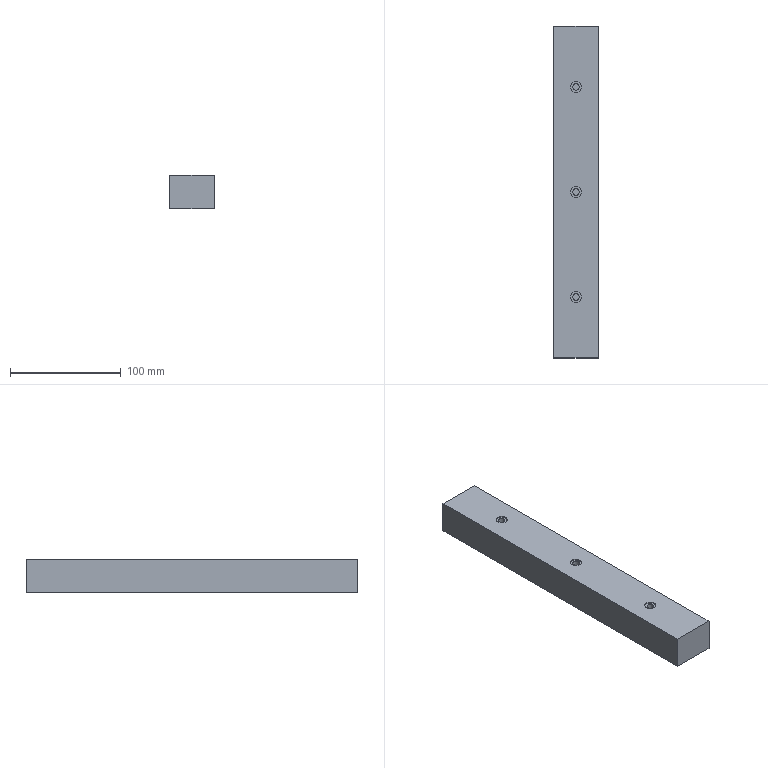Part | STEP file | lizhu | 1 solid | 18 faces | box 40 x 300 x 30 mm | volume 358407 mm3 | plane 12 | cylinder 6 | commonest cylinder face diameters 6 x3 10 x3
STEP:
#1=CARTESIAN_POINT('',(0.,0.,0.));
#2=DIRECTION('',(0.,0.,1.));
#3=DIRECTION('',(1.,0.,0.));
#4=AXIS2_PLACEMENT_3D('',#1,#2,#3);
#5=CARTESIAN_POINT('',(20.,-150.,0.));
#6=VERTEX_POINT('',#5);
#7=CARTESIAN_POINT('',(20.,150.,0.));
#8=VERTEX_POINT('',#7);
#9=CARTESIAN_POINT('',(20.,150.,0.));
#10=DIRECTION('',(0.,1.,0.));
#11=VECTOR('',#10,1.);
#12=LINE('',#9,#11);
#13=CARTESIAN_POINT('',(20.,150.,30.));
#14=DIRECTION('',(-1.,0.,0.));
#15=DIRECTION('',(0.,-1.,0.));
#16=AXIS2_PLACEMENT_3D('',#13,#14,#15);
#17=PLANE('',#16);
#18=CARTESIAN_POINT('',(0.,-30.));
#19=DIRECTION('',(-1.,0.));
#20=VECTOR('',#19,1.);
#21=LINE('',#18,#20);
#22=(GEOMETRIC_REPRESENTATION_CONTEXT(2)PARAMETRIC_REPRESENTATION_CONTEXT()REPRESENTATION_CONTEXT('',''));
#23=DEFINITIONAL_REPRESENTATION('',(#21),#22);
#24=PCURVE('',#17,#23);
#25=CARTESIAN_POINT('',(0.,0.,0.));
#26=DIRECTION('',(0.,0.,1.));
#27=DIRECTION('',(1.,0.,0.));
#28=AXIS2_PLACEMENT_3D('',#25,#26,#27);
#29=PLANE('',#28);
#30=CARTESIAN_POINT('',(20.,150.));
#31=DIRECTION('',(0.,1.));
#32=VECTOR('',#31,1.);
#33=LINE('',#30,#32);
#34=(GEOMETRIC_REPRESENTATION_CONTEXT(2)PARAMETRIC_REPRESENTATION_CONTEXT()REPRESENTATION_CONTEXT('',''));
#35=DEFINITIONAL_REPRESENTATION('',(#33),#34);
#36=PCURVE('',#29,#35);
#37=SURFACE_CURVE('',#12,(#24,#36),.PCURVE_S1.);
#38=EDGE_CURVE('',#6,#8,#37,.T.);
#39=ORIENTED_EDGE('',*,*,#38,.T.);
#40=CARTESIAN_POINT('',(20.,150.,30.));
#41=VERTEX_POINT('',#40);
#42=CARTESIAN_POINT('',(20.,150.,30.));
#43=DIRECTION('',(0.,0.,-1.));
#44=VECTOR('',#43,1.);
#45=LINE('',#42,#44);
#46=CARTESIAN_POINT('',(0.,0.));
#47=DIRECTION('',(0.,-1.));
#48=VECTOR('',#47,1.);
#49=LINE('',#46,#48);
#50=(GEOMETRIC_REPRESENTATION_CONTEXT(2)PARAMETRIC_REPRESENTATION_CONTEXT()REPRESENTATION_CONTEXT('',''));
#51=DEFINITIONAL_REPRESENTATION('',(#49),#50);
#52=PCURVE('',#17,#51);
#53=CARTESIAN_POINT('',(-20.,150.,30.));
#54=DIRECTION('',(0.,-1.,0.));
#55=DIRECTION('',(0.,0.,-1.));
#56=AXIS2_PLACEMENT_3D('',#53,#54,#55);
#57=PLANE('',#56);
#58=CARTESIAN_POINT('',(0.,40.));
#59=DIRECTION('',(1.,0.));
#60=VECTOR('',#59,1.);
#61=LINE('',#58,#60);
#62=(GEOMETRIC_REPRESENTATION_CONTEXT(2)PARAMETRIC_REPRESENTATION_CONTEXT()REPRESENTATION_CONTEXT('',''));
#63=DEFINITIONAL_REPRESENTATION('',(#61),#62);
#64=PCURVE('',#57,#63);
#65=SURFACE_CURVE('',#45,(#52,#64),.PCURVE_S1.);
#66=EDGE_CURVE('',#41,#8,#65,.T.);
#67=ORIENTED_EDGE('',*,*,#66,.F.);
#68=CARTESIAN_POINT('',(20.,-150.,30.));
#69=VERTEX_POINT('',#68);
#70=CARTESIAN_POINT('',(20.,150.,30.));
#71=DIRECTION('',(0.,1.,0.));
#72=VECTOR('',#71,1.);
#73=LINE('',#70,#72);
#74=CARTESIAN_POINT('',(0.,0.));
#75=DIRECTION('',(-1.,0.));
#76=VECTOR('',#75,1.);
#77=LINE('',#74,#76);
#78=(GEOMETRIC_REPRESENTATION_CONTEXT(2)PARAMETRIC_REPRESENTATION_CONTEXT()REPRESENTATION_CONTEXT('',''));
#79=DEFINITIONAL_REPRESENTATION('',(#77),#78);
#80=PCURVE('',#17,#79);
#81=CARTESIAN_POINT('',(0.,0.,30.));
#82=DIRECTION('',(0.,0.,1.));
#83=DIRECTION('',(1.,0.,0.));
#84=AXIS2_PLACEMENT_3D('',#81,#82,#83);
#85=PLANE('',#84);
#86=CARTESIAN_POINT('',(20.,150.));
#87=DIRECTION('',(0.,1.));
#88=VECTOR('',#87,1.);
#89=LINE('',#86,#88);
#90=(GEOMETRIC_REPRESENTATION_CONTEXT(2)PARAMETRIC_REPRESENTATION_CONTEXT()REPRESENTATION_CONTEXT('',''));
#91=DEFINITIONAL_REPRESENTATION('',(#89),#90);
#92=PCURVE('',#85,#91);
#93=SURFACE_CURVE('',#73,(#80,#92),.PCURVE_S1.);
#94=EDGE_CURVE('',#69,#41,#93,.T.);
#95=ORIENTED_EDGE('',*,*,#94,.F.);
#96=CARTESIAN_POINT('',(20.,-150.,30.));
#97=DIRECTION('',(0.,0.,-1.));
#98=VECTOR('',#97,1.);
#99=LINE('',#96,#98);
#100=CARTESIAN_POINT('',(300.,0.));
#101=DIRECTION('',(0.,-1.));
#102=VECTOR('',#101,1.);
#103=LINE('',#100,#102);
#104=(GEOMETRIC_REPRESENTATION_CONTEXT(2)PARAMETRIC_REPRESENTATION_CONTEXT()REPRESENTATION_CONTEXT('',''));
#105=DEFINITIONAL_REPRESENTATION('',(#103),#104);
#106=PCURVE('',#17,#105);
#107=CARTESIAN_POINT('',(-20.,-150.,30.));
#108=DIRECTION('',(0.,1.,0.));
#109=DIRECTION('',(0.,0.,1.));
#110=AXIS2_PLACEMENT_3D('',#107,#108,#109);
#111=PLANE('',#110);
#112=CARTESIAN_POINT('',(0.,40.));
#113=DIRECTION('',(-1.,0.));
#114=VECTOR('',#113,1.);
#115=LINE('',#112,#114);
#116=(GEOMETRIC_REPRESENTATION_CONTEXT(2)PARAMETRIC_REPRESENTATION_CONTEXT()REPRESENTATION_CONTEXT('',''));
#117=DEFINITIONAL_REPRESENTATION('',(#115),#116);
#118=PCURVE('',#111,#117);
#119=SURFACE_CURVE('',#99,(#106,#118),.PCURVE_S1.);
#120=EDGE_CURVE('',#69,#6,#119,.T.);
#121=ORIENTED_EDGE('',*,*,#120,.T.);
#122=EDGE_LOOP('',(#39,#67,#95,#121));
#123=FACE_BOUND('',#122,.T.);
#124=ADVANCED_FACE('',(#123),#17,.F.);
#125=CARTESIAN_POINT('',(-20.,150.,0.));
#126=VERTEX_POINT('',#125);
#127=CARTESIAN_POINT('',(-20.,150.,0.));
#128=DIRECTION('',(-1.,0.,0.));
#129=VECTOR('',#128,1.);
#130=LINE('',#127,#129);
#131=CARTESIAN_POINT('',(30.,0.));
#132=DIRECTION('',(0.,-1.));
#133=VECTOR('',#132,1.);
#134=LINE('',#131,#133);
#135=(GEOMETRIC_REPRESENTATION_CONTEXT(2)PARAMETRIC_REPRESENTATION_CONTEXT()REPRESENTATION_CONTEXT('',''));
#136=DEFINITIONAL_REPRESENTATION('',(#134),#135);
#137=PCURVE('',#57,#136);
#138=CARTESIAN_POINT('',(-20.,150.));
#139=DIRECTION('',(-1.,0.));
#140=VECTOR('',#139,1.);
#141=LINE('',#138,#140);
#142=(GEOMETRIC_REPRESENTATION_CONTEXT(2)PARAMETRIC_REPRESENTATION_CONTEXT()REPRESENTATION_CONTEXT('',''));
#143=DEFINITIONAL_REPRESENTATION('',(#141),#142);
#144=PCURVE('',#29,#143);
#145=SURFACE_CURVE('',#130,(#137,#144),.PCURVE_S1.);
#146=EDGE_CURVE('',#8,#126,#145,.T.);
#147=ORIENTED_EDGE('',*,*,#146,.T.);
#148=CARTESIAN_POINT('',(-20.,150.,30.));
#149=VERTEX_POINT('',#148);
#150=CARTESIAN_POINT('',(-20.,150.,30.));
#151=DIRECTION('',(0.,0.,-1.));
#152=VECTOR('',#151,1.);
#153=LINE('',#150,#152);
#154=CARTESIAN_POINT('',(0.,0.));
#155=DIRECTION('',(1.,0.));
#156=VECTOR('',#155,1.);
#157=LINE('',#154,#156);
#158=(GEOMETRIC_REPRESENTATION_CONTEXT(2)PARAMETRIC_REPRESENTATION_CONTEXT()REPRESENTATION_CONTEXT('',''));
#159=DEFINITIONAL_REPRESENTATION('',(#157),#158);
#160=PCURVE('',#57,#159);
#161=CARTESIAN_POINT('',(-20.,150.,30.));
#162=DIRECTION('',(1.,0.,0.));
#163=DIRECTION('',(0.,1.,0.));
#164=AXIS2_PLACEMENT_3D('',#161,#162,#163);
#165=PLANE('',#164);
#166=CARTESIAN_POINT('',(0.,0.));
#167=DIRECTION('',(0.,-1.));
#168=VECTOR('',#167,1.);
#169=LINE('',#166,#168);
#170=(GEOMETRIC_REPRESENTATION_CONTEXT(2)PARAMETRIC_REPRESENTATION_CONTEXT()REPRESENTATION_CONTEXT('',''));
#171=DEFINITIONAL_REPRESENTATION('',(#169),#170);
#172=PCURVE('',#165,#171);
#173=SURFACE_CURVE('',#153,(#160,#172),.PCURVE_S1.);
#174=EDGE_CURVE('',#149,#126,#173,.T.);
#175=ORIENTED_EDGE('',*,*,#174,.F.);
#176=CARTESIAN_POINT('',(-20.,150.,30.));
#177=DIRECTION('',(-1.,0.,0.));
#178=VECTOR('',#177,1.);
#179=LINE('',#176,#178);
#180=CARTESIAN_POINT('',(0.,0.));
#181=DIRECTION('',(0.,-1.));
#182=VECTOR('',#181,1.);
#183=LINE('',#180,#182);
#184=(GEOMETRIC_REPRESENTATION_CONTEXT(2)PARAMETRIC_REPRESENTATION_CONTEXT()REPRESENTATION_CONTEXT('',''));
#185=DEFINITIONAL_REPRESENTATION('',(#183),#184);
#186=PCURVE('',#57,#185);
#187=CARTESIAN_POINT('',(-20.,150.));
#188=DIRECTION('',(-1.,0.));
#189=VECTOR('',#188,1.);
#190=LINE('',#187,#189);
#191=(GEOMETRIC_REPRESENTATION_CONTEXT(2)PARAMETRIC_REPRESENTATION_CONTEXT()REPRESENTATION_CONTEXT('',''));
#192=DEFINITIONAL_REPRESENTATION('',(#190),#191);
#193=PCURVE('',#85,#192);
#194=SURFACE_CURVE('',#179,(#186,#193),.PCURVE_S1.);
#195=EDGE_CURVE('',#41,#149,#194,.T.);
#196=ORIENTED_EDGE('',*,*,#195,.F.);
#197=ORIENTED_EDGE('',*,*,#66,.T.);
#198=EDGE_LOOP('',(#147,#175,#196,#197));
#199=FACE_BOUND('',#198,.T.);
#200=ADVANCED_FACE('',(#199),#57,.F.);
#201=CARTESIAN_POINT('',(-20.,-150.,0.));
#202=VERTEX_POINT('',#201);
#203=CARTESIAN_POINT('',(-20.,150.,0.));
#204=DIRECTION('',(0.,-1.,0.));
#205=VECTOR('',#204,1.);
#206=LINE('',#203,#205);
#207=CARTESIAN_POINT('',(0.,-30.));
#208=DIRECTION('',(-1.,0.));
#209=VECTOR('',#208,1.);
#210=LINE('',#207,#209);
#211=(GEOMETRIC_REPRESENTATION_CONTEXT(2)PARAMETRIC_REPRESENTATION_CONTEXT()REPRESENTATION_CONTEXT('',''));
#212=DEFINITIONAL_REPRESENTATION('',(#210),#211);
#213=PCURVE('',#165,#212);
#214=CARTESIAN_POINT('',(-20.,150.));
#215=DIRECTION('',(0.,-1.));
#216=VECTOR('',#215,1.);
#217=LINE('',#214,#216);
#218=(GEOMETRIC_REPRESENTATION_CONTEXT(2)PARAMETRIC_REPRESENTATION_CONTEXT()REPRESENTATION_CONTEXT('',''));
#219=DEFINITIONAL_REPRESENTATION('',(#217),#218);
#220=PCURVE('',#29,#219);
#221=SURFACE_CURVE('',#206,(#213,#220),.PCURVE_S1.);
#222=EDGE_CURVE('',#126,#202,#221,.T.);
#223=ORIENTED_EDGE('',*,*,#222,.T.);
#224=CARTESIAN_POINT('',(-20.,-150.,30.));
#225=VERTEX_POINT('',#224);
#226=CARTESIAN_POINT('',(-20.,-150.,30.));
#227=DIRECTION('',(0.,0.,-1.));
#228=VECTOR('',#227,1.);
#229=LINE('',#226,#228);
#230=CARTESIAN_POINT('',(-300.,0.));
#231=DIRECTION('',(0.,-1.));
#232=VECTOR('',#231,1.);
#233=LINE('',#230,#232);
#234=(GEOMETRIC_REPRESENTATION_CONTEXT(2)PARAMETRIC_REPRESENTATION_CONTEXT()REPRESENTATION_CONTEXT('',''));
#235=DEFINITIONAL_REPRESENTATION('',(#233),#234);
#236=PCURVE('',#165,#235);
#237=CARTESIAN_POINT('',(0.,0.));
#238=DIRECTION('',(-1.,0.));
#239=VECTOR('',#238,1.);
#240=LINE('',#237,#239);
#241=(GEOMETRIC_REPRESENTATION_CONTEXT(2)PARAMETRIC_REPRESENTATION_CONTEXT()REPRESENTATION_CONTEXT('',''));
#242=DEFINITIONAL_REPRESENTATION('',(#240),#241);
#243=PCURVE('',#111,#242);
#244=SURFACE_CURVE('',#229,(#236,#243),.PCURVE_S1.);
#245=EDGE_CURVE('',#225,#202,#244,.T.);
#246=ORIENTED_EDGE('',*,*,#245,.F.);
#247=CARTESIAN_POINT('',(-20.,150.,30.));
#248=DIRECTION('',(0.,-1.,0.));
#249=VECTOR('',#248,1.);
#250=LINE('',#247,#249);
#251=CARTESIAN_POINT('',(0.,0.));
#252=DIRECTION('',(-1.,0.));
#253=VECTOR('',#252,1.);
#254=LINE('',#251,#253);
#255=(GEOMETRIC_REPRESENTATION_CONTEXT(2)PARAMETRIC_REPRESENTATION_CONTEXT()REPRESENTATION_CONTEXT('',''));
#256=DEFINITIONAL_REPRESENTATION('',(#254),#255);
#257=PCURVE('',#165,#256);
#258=CARTESIAN_POINT('',(-20.,150.));
#259=DIRECTION('',(0.,-1.));
#260=VECTOR('',#259,1.);
#261=LINE('',#258,#260);
#262=(GEOMETRIC_REPRESENTATION_CONTEXT(2)PARAMETRIC_REPRESENTATION_CONTEXT()REPRESENTATION_CONTEXT('',''));
#263=DEFINITIONAL_REPRESENTATION('',(#261),#262);
#264=PCURVE('',#85,#263);
#265=SURFACE_CURVE('',#250,(#257,#264),.PCURVE_S1.);
#266=EDGE_CURVE('',#149,#225,#265,.T.);
#267=ORIENTED_EDGE('',*,*,#266,.F.);
#268=ORIENTED_EDGE('',*,*,#174,.T.);
#269=EDGE_LOOP('',(#223,#246,#267,#268));
#270=FACE_BOUND('',#269,.T.);
#271=ADVANCED_FACE('',(#270),#165,.F.);
#272=CARTESIAN_POINT('',(-20.,-150.,0.));
#273=DIRECTION('',(1.,0.,0.));
#274=VECTOR('',#273,1.);
#275=LINE('',#272,#274);
#276=CARTESIAN_POINT('',(-30.,0.));
#277=DIRECTION('',(0.,1.));
#278=VECTOR('',#277,1.);
#279=LINE('',#276,#278);
#280=(GEOMETRIC_REPRESENTATION_CONTEXT(2)PARAMETRIC_REPRESENTATION_CONTEXT()REPRESENTATION_CONTEXT('',''));
#281=DEFINITIONAL_REPRESENTATION('',(#279),#280);
#282=PCURVE('',#111,#281);
#283=CARTESIAN_POINT('',(-20.,-150.));
#284=DIRECTION('',(1.,0.));
#285=VECTOR('',#284,1.);
#286=LINE('',#283,#285);
#287=(GEOMETRIC_REPRESENTATION_CONTEXT(2)PARAMETRIC_REPRESENTATION_CONTEXT()REPRESENTATION_CONTEXT('',''));
#288=DEFINITIONAL_REPRESENTATION('',(#286),#287);
#289=PCURVE('',#29,#288);
#290=SURFACE_CURVE('',#275,(#282,#289),.PCURVE_S1.);
#291=EDGE_CURVE('',#202,#6,#290,.T.);
#292=ORIENTED_EDGE('',*,*,#291,.T.);
#293=ORIENTED_EDGE('',*,*,#120,.F.);
#294=CARTESIAN_POINT('',(-20.,-150.,30.));
#295=DIRECTION('',(1.,0.,0.));
#296=VECTOR('',#295,1.);
#297=LINE('',#294,#296);
#298=CARTESIAN_POINT('',(0.,0.));
#299=DIRECTION('',(0.,1.));
#300=VECTOR('',#299,1.);
#301=LINE('',#298,#300);
#302=(GEOMETRIC_REPRESENTATION_CONTEXT(2)PARAMETRIC_REPRESENTATION_CONTEXT()REPRESENTATION_CONTEXT('',''));
#303=DEFINITIONAL_REPRESENTATION('',(#301),#302);
#304=PCURVE('',#111,#303);
#305=CARTESIAN_POINT('',(-20.,-150.));
#306=DIRECTION('',(1.,0.));
#307=VECTOR('',#306,1.);
#308=LINE('',#305,#307);
#309=(GEOMETRIC_REPRESENTATION_CONTEXT(2)PARAMETRIC_REPRESENTATION_CONTEXT()REPRESENTATION_CONTEXT('',''));
#310=DEFINITIONAL_REPRESENTATION('',(#308),#309);
#311=PCURVE('',#85,#310);
#312=SURFACE_CURVE('',#297,(#304,#311),.PCURVE_S1.);
#313=EDGE_CURVE('',#225,#69,#312,.T.);
#314=ORIENTED_EDGE('',*,*,#313,.F.);
#315=ORIENTED_EDGE('',*,*,#245,.T.);
#316=EDGE_LOOP('',(#292,#293,#314,#315));
#317=FACE_BOUND('',#316,.T.);
#318=ADVANCED_FACE('',(#317),#111,.F.);
#319=CARTESIAN_POINT('',(5.,95.,30.));
#320=VERTEX_POINT('',#319);
#321=CARTESIAN_POINT('',(0.,95.,30.));
#322=DIRECTION('',(0.,0.,1.));
#323=DIRECTION('',(1.,0.,0.));
#324=AXIS2_PLACEMENT_3D('',#321,#322,#323);
#325=CIRCLE('',#324,5.);
#326=CARTESIAN_POINT('',(0.,95.));
#327=DIRECTION('',(1.,0.));
#328=AXIS2_PLACEMENT_2D('',#326,#327);
#329=CIRCLE('',#328,5.);
#330=(GEOMETRIC_REPRESENTATION_CONTEXT(2)PARAMETRIC_REPRESENTATION_CONTEXT()REPRESENTATION_CONTEXT('',''));
#331=DEFINITIONAL_REPRESENTATION('',(#329),#330);
#332=PCURVE('',#85,#331);
#333=CARTESIAN_POINT('',(0.,95.,29.));
#334=DIRECTION('',(0.,0.,1.));
#335=DIRECTION('',(1.,0.,0.));
#336=AXIS2_PLACEMENT_3D('',#333,#334,#335);
#337=CYLINDRICAL_SURFACE('',#336,5.);
#338=CARTESIAN_POINT('',(0.,1.));
#339=DIRECTION('',(1.,0.));
#340=VECTOR('',#339,1.);
#341=LINE('',#338,#340);
#342=(GEOMETRIC_REPRESENTATION_CONTEXT(2)PARAMETRIC_REPRESENTATION_CONTEXT()REPRESENTATION_CONTEXT('',''));
#343=DEFINITIONAL_REPRESENTATION('',(#341),#342);
#344=PCURVE('',#337,#343);
#345=SURFACE_CURVE('',#325,(#332,#344),.PCURVE_S1.);
#346=EDGE_CURVE('',#320,#320,#345,.T.);
#347=ORIENTED_EDGE('',*,*,#346,.F.);
#348=EDGE_LOOP('',(#347));
#349=FACE_BOUND('',#348,.T.);
#350=CARTESIAN_POINT('',(5.,-95.,30.));
#351=VERTEX_POINT('',#350);
#352=CARTESIAN_POINT('',(0.,-95.,30.));
#353=DIRECTION('',(0.,0.,1.));
#354=DIRECTION('',(1.,0.,0.));
#355=AXIS2_PLACEMENT_3D('',#352,#353,#354);
#356=CIRCLE('',#355,5.);
#357=CARTESIAN_POINT('',(0.,-95.));
#358=DIRECTION('',(1.,0.));
#359=AXIS2_PLACEMENT_2D('',#357,#358);
#360=CIRCLE('',#359,5.);
#361=(GEOMETRIC_REPRESENTATION_CONTEXT(2)PARAMETRIC_REPRESENTATION_CONTEXT()REPRESENTATION_CONTEXT('',''));
#362=DEFINITIONAL_REPRESENTATION('',(#360),#361);
#363=PCURVE('',#85,#362);
#364=CARTESIAN_POINT('',(0.,-95.,29.));
#365=DIRECTION('',(0.,0.,1.));
#366=DIRECTION('',(1.,0.,0.));
#367=AXIS2_PLACEMENT_3D('',#364,#365,#366);
#368=CYLINDRICAL_SURFACE('',#367,5.);
#369=CARTESIAN_POINT('',(0.,1.));
#370=DIRECTION('',(1.,0.));
#371=VECTOR('',#370,1.);
#372=LINE('',#369,#371);
#373=(GEOMETRIC_REPRESENTATION_CONTEXT(2)PARAMETRIC_REPRESENTATION_CONTEXT()REPRESENTATION_CONTEXT('',''));
#374=DEFINITIONAL_REPRESENTATION('',(#372),#373);
#375=PCURVE('',#368,#374);
#376=SURFACE_CURVE('',#356,(#363,#375),.PCURVE_S1.);
#377=EDGE_CURVE('',#351,#351,#376,.T.);
#378=ORIENTED_EDGE('',*,*,#377,.F.);
#379=EDGE_LOOP('',(#378));
#380=FACE_BOUND('',#379,.T.);
#381=CARTESIAN_POINT('',(5.,0.,30.));
#382=VERTEX_POINT('',#381);
#383=CARTESIAN_POINT('',(0.,0.,30.));
#384=DIRECTION('',(0.,0.,1.));
#385=DIRECTION('',(1.,0.,0.));
#386=AXIS2_PLACEMENT_3D('',#383,#384,#385);
#387=CIRCLE('',#386,5.);
#388=CARTESIAN_POINT('',(0.,0.));
#389=DIRECTION('',(1.,0.));
#390=AXIS2_PLACEMENT_2D('',#388,#389);
#391=CIRCLE('',#390,5.);
#392=(GEOMETRIC_REPRESENTATION_CONTEXT(2)PARAMETRIC_REPRESENTATION_CONTEXT()REPRESENTATION_CONTEXT('',''));
#393=DEFINITIONAL_REPRESENTATION('',(#391),#392);
#394=PCURVE('',#85,#393);
#395=CARTESIAN_POINT('',(0.,0.,29.));
#396=DIRECTION('',(0.,0.,1.));
#397=DIRECTION('',(1.,0.,0.));
#398=AXIS2_PLACEMENT_3D('',#395,#396,#397);
#399=CYLINDRICAL_SURFACE('',#398,5.);
#400=CARTESIAN_POINT('',(0.,1.));
#401=DIRECTION('',(1.,0.));
#402=VECTOR('',#401,1.);
#403=LINE('',#400,#402);
#404=(GEOMETRIC_REPRESENTATION_CONTEXT(2)PARAMETRIC_REPRESENTATION_CONTEXT()REPRESENTATION_CONTEXT('',''));
#405=DEFINITIONAL_REPRESENTATION('',(#403),#404);
#406=PCURVE('',#399,#405);
#407=SURFACE_CURVE('',#387,(#394,#406),.PCURVE_S1.);
#408=EDGE_CURVE('',#382,#382,#407,.T.);
#409=ORIENTED_EDGE('',*,*,#408,.F.);
#410=EDGE_LOOP('',(#409));
#411=FACE_BOUND('',#410,.T.);
#412=ORIENTED_EDGE('',*,*,#94,.T.);
#413=ORIENTED_EDGE('',*,*,#195,.T.);
#414=ORIENTED_EDGE('',*,*,#266,.T.);
#415=ORIENTED_EDGE('',*,*,#313,.T.);
#416=EDGE_LOOP('',(#412,#413,#414,#415));
#417=FACE_BOUND('',#416,.T.);
#418=ADVANCED_FACE('',(#349,#380,#411,#417),#85,.T.);
#419=ORIENTED_EDGE('',*,*,#38,.F.);
#420=ORIENTED_EDGE('',*,*,#291,.F.);
#421=ORIENTED_EDGE('',*,*,#222,.F.);
#422=ORIENTED_EDGE('',*,*,#146,.F.);
#423=EDGE_LOOP('',(#419,#420,#421,#422));
#424=FACE_BOUND('',#423,.T.);
#425=ADVANCED_FACE('',(#424),#29,.F.);
#426=CARTESIAN_POINT('',(5.,0.,29.));
#427=VERTEX_POINT('',#426);
#428=CARTESIAN_POINT('',(0.,0.,29.));
#429=DIRECTION('',(0.,0.,1.));
#430=DIRECTION('',(1.,0.,0.));
#431=AXIS2_PLACEMENT_3D('',#428,#429,#430);
#432=CIRCLE('',#431,5.);
#433=CARTESIAN_POINT('',(0.,0.));
#434=DIRECTION('',(1.,0.));
#435=VECTOR('',#434,1.);
#436=LINE('',#433,#435);
#437=(GEOMETRIC_REPRESENTATION_CONTEXT(2)PARAMETRIC_REPRESENTATION_CONTEXT()REPRESENTATION_CONTEXT('',''));
#438=DEFINITIONAL_REPRESENTATION('',(#436),#437);
#439=PCURVE('',#399,#438);
#440=CARTESIAN_POINT('',(0.,0.,29.));
#441=DIRECTION('',(0.,0.,1.));
#442=DIRECTION('',(1.,0.,0.));
#443=AXIS2_PLACEMENT_3D('',#440,#441,#442);
#444=PLANE('',#443);
#445=CARTESIAN_POINT('',(0.,0.));
#446=DIRECTION('',(1.,0.));
#447=AXIS2_PLACEMENT_2D('',#445,#446);
#448=CIRCLE('',#447,5.);
#449=(GEOMETRIC_REPRESENTATION_CONTEXT(2)PARAMETRIC_REPRESENTATION_CONTEXT()REPRESENTATION_CONTEXT('',''));
#450=DEFINITIONAL_REPRESENTATION('',(#448),#449);
#451=PCURVE('',#444,#450);
#452=SURFACE_CURVE('',#432,(#439,#451),.PCURVE_S1.);
#453=EDGE_CURVE('',#427,#427,#452,.T.);
#454=ORIENTED_EDGE('',*,*,#453,.T.);
#455=CARTESIAN_POINT('',(5.,0.,29.));
#456=CARTESIAN_POINT('',(5.,0.,30.));
#457=B_SPLINE_CURVE_WITH_KNOTS('',1,(#455,#456),.UNSPECIFIED.,.F.,.F.,(2,2),(0.,1.),.PIECEWISE_BEZIER_KNOTS.);
#458=CARTESIAN_POINT('',(6.283,0.));
#459=DIRECTION('',(0.,1.));
#460=VECTOR('',#459,1.);
#461=LINE('',#458,#460);
#462=(GEOMETRIC_REPRESENTATION_CONTEXT(2)PARAMETRIC_REPRESENTATION_CONTEXT()REPRESENTATION_CONTEXT('',''));
#463=DEFINITIONAL_REPRESENTATION('',(#461),#462);
#464=PCURVE('',#399,#463);
#465=CARTESIAN_POINT('',(0.,0.));
#466=DIRECTION('',(0.,1.));
#467=VECTOR('',#466,1.);
#468=LINE('',#465,#467);
#469=(GEOMETRIC_REPRESENTATION_CONTEXT(2)PARAMETRIC_REPRESENTATION_CONTEXT()REPRESENTATION_CONTEXT('',''));
#470=DEFINITIONAL_REPRESENTATION('',(#468),#469);
#471=PCURVE('',#399,#470);
#472=SEAM_CURVE('',#457,(#464,#471),.PCURVE_S1.);
#473=EDGE_CURVE('',#427,#382,#472,.T.);
#474=ORIENTED_EDGE('',*,*,#473,.T.);
#475=ORIENTED_EDGE('',*,*,#408,.F.);
#476=ORIENTED_EDGE('',*,*,#473,.F.);
#477=EDGE_LOOP('',(#454,#474,#475,#476));
#478=FACE_BOUND('',#477,.F.);
#479=ADVANCED_FACE('',(#478),#399,.F.);
#480=CARTESIAN_POINT('',(3.,0.,29.));
#481=VERTEX_POINT('',#480);
#482=CARTESIAN_POINT('',(0.,0.,29.));
#483=DIRECTION('',(0.,0.,1.));
#484=DIRECTION('',(1.,0.,0.));
#485=AXIS2_PLACEMENT_3D('',#482,#483,#484);
#486=CIRCLE('',#485,3.);
#487=CARTESIAN_POINT('',(0.,0.));
#488=DIRECTION('',(1.,0.));
#489=AXIS2_PLACEMENT_2D('',#487,#488);
#490=CIRCLE('',#489,3.);
#491=(GEOMETRIC_REPRESENTATION_CONTEXT(2)PARAMETRIC_REPRESENTATION_CONTEXT()REPRESENTATION_CONTEXT('',''));
#492=DEFINITIONAL_REPRESENTATION('',(#490),#491);
#493=PCURVE('',#444,#492);
#494=CARTESIAN_POINT('',(0.,0.,13.));
#495=DIRECTION('',(0.,0.,1.));
#496=DIRECTION('',(1.,0.,0.));
#497=AXIS2_PLACEMENT_3D('',#494,#495,#496);
#498=CYLINDRICAL_SURFACE('',#497,3.);
#499=CARTESIAN_POINT('',(0.,16.));
#500=DIRECTION('',(1.,0.));
#501=VECTOR('',#500,1.);
#502=LINE('',#499,#501);
#503=(GEOMETRIC_REPRESENTATION_CONTEXT(2)PARAMETRIC_REPRESENTATION_CONTEXT()REPRESENTATION_CONTEXT('',''));
#504=DEFINITIONAL_REPRESENTATION('',(#502),#503);
#505=PCURVE('',#498,#504);
#506=SURFACE_CURVE('',#486,(#493,#505),.PCURVE_S1.);
#507=EDGE_CURVE('',#481,#481,#506,.T.);
#508=ORIENTED_EDGE('',*,*,#507,.F.);
#509=EDGE_LOOP('',(#508));
#510=FACE_BOUND('',#509,.T.);
#511=ORIENTED_EDGE('',*,*,#453,.T.);
#512=EDGE_LOOP('',(#511));
#513=FACE_BOUND('',#512,.T.);
#514=ADVANCED_FACE('',(#510,#513),#444,.T.);
#515=CARTESIAN_POINT('',(5.,-95.,29.));
#516=VERTEX_POINT('',#515);
#517=CARTESIAN_POINT('',(0.,-95.,29.));
#518=DIRECTION('',(0.,0.,1.));
#519=DIRECTION('',(1.,0.,0.));
#520=AXIS2_PLACEMENT_3D('',#517,#518,#519);
#521=CIRCLE('',#520,5.);
#522=CARTESIAN_POINT('',(0.,0.));
#523=DIRECTION('',(1.,0.));
#524=VECTOR('',#523,1.);
#525=LINE('',#522,#524);
#526=(GEOMETRIC_REPRESENTATION_CONTEXT(2)PARAMETRIC_REPRESENTATION_CONTEXT()REPRESENTATION_CONTEXT('',''));
#527=DEFINITIONAL_REPRESENTATION('',(#525),#526);
#528=PCURVE('',#368,#527);
#529=CARTESIAN_POINT('',(0.,-95.,29.));
#530=DIRECTION('',(0.,0.,1.));
#531=DIRECTION('',(1.,0.,0.));
#532=AXIS2_PLACEMENT_3D('',#529,#530,#531);
#533=PLANE('',#532);
#534=CARTESIAN_POINT('',(0.,0.));
#535=DIRECTION('',(1.,0.));
#536=AXIS2_PLACEMENT_2D('',#534,#535);
#537=CIRCLE('',#536,5.);
#538=(GEOMETRIC_REPRESENTATION_CONTEXT(2)PARAMETRIC_REPRESENTATION_CONTEXT()REPRESENTATION_CONTEXT('',''));
#539=DEFINITIONAL_REPRESENTATION('',(#537),#538);
#540=PCURVE('',#533,#539);
#541=SURFACE_CURVE('',#521,(#528,#540),.PCURVE_S1.);
#542=EDGE_CURVE('',#516,#516,#541,.T.);
#543=ORIENTED_EDGE('',*,*,#542,.T.);
#544=CARTESIAN_POINT('',(5.,-95.,29.));
#545=CARTESIAN_POINT('',(5.,-95.,30.));
#546=B_SPLINE_CURVE_WITH_KNOTS('',1,(#544,#545),.UNSPECIFIED.,.F.,.F.,(2,2),(0.,1.),.PIECEWISE_BEZIER_KNOTS.);
#547=CARTESIAN_POINT('',(6.283,0.));
#548=DIRECTION('',(0.,1.));
#549=VECTOR('',#548,1.);
#550=LINE('',#547,#549);
#551=(GEOMETRIC_REPRESENTATION_CONTEXT(2)PARAMETRIC_REPRESENTATION_CONTEXT()REPRESENTATION_CONTEXT('',''));
#552=DEFINITIONAL_REPRESENTATION('',(#550),#551);
#553=PCURVE('',#368,#552);
#554=CARTESIAN_POINT('',(0.,0.));
#555=DIRECTION('',(0.,1.));
#556=VECTOR('',#555,1.);
#557=LINE('',#554,#556);
#558=(GEOMETRIC_REPRESENTATION_CONTEXT(2)PARAMETRIC_REPRESENTATION_CONTEXT()REPRESENTATION_CONTEXT('',''));
#559=DEFINITIONAL_REPRESENTATION('',(#557),#558);
#560=PCURVE('',#368,#559);
#561=SEAM_CURVE('',#546,(#553,#560),.PCURVE_S1.);
#562=EDGE_CURVE('',#516,#351,#561,.T.);
#563=ORIENTED_EDGE('',*,*,#562,.T.);
#564=ORIENTED_EDGE('',*,*,#377,.F.);
#565=ORIENTED_EDGE('',*,*,#562,.F.);
#566=EDGE_LOOP('',(#543,#563,#564,#565));
#567=FACE_BOUND('',#566,.F.);
#568=ADVANCED_FACE('',(#567),#368,.F.);
#569=CARTESIAN_POINT('',(3.,-95.,29.));
#570=VERTEX_POINT('',#569);
#571=CARTESIAN_POINT('',(0.,-95.,29.));
#572=DIRECTION('',(0.,0.,1.));
#573=DIRECTION('',(1.,0.,0.));
#574=AXIS2_PLACEMENT_3D('',#571,#572,#573);
#575=CIRCLE('',#574,3.);
#576=CARTESIAN_POINT('',(0.,0.));
#577=DIRECTION('',(1.,0.));
#578=AXIS2_PLACEMENT_2D('',#576,#577);
#579=CIRCLE('',#578,3.);
#580=(GEOMETRIC_REPRESENTATION_CONTEXT(2)PARAMETRIC_REPRESENTATION_CONTEXT()REPRESENTATION_CONTEXT('',''));
#581=DEFINITIONAL_REPRESENTATION('',(#579),#580);
#582=PCURVE('',#533,#581);
#583=CARTESIAN_POINT('',(0.,-95.,13.));
#584=DIRECTION('',(0.,0.,1.));
#585=DIRECTION('',(1.,0.,0.));
#586=AXIS2_PLACEMENT_3D('',#583,#584,#585);
#587=CYLINDRICAL_SURFACE('',#586,3.);
#588=CARTESIAN_POINT('',(0.,16.));
#589=DIRECTION('',(1.,0.));
#590=VECTOR('',#589,1.);
#591=LINE('',#588,#590);
#592=(GEOMETRIC_REPRESENTATION_CONTEXT(2)PARAMETRIC_REPRESENTATION_CONTEXT()REPRESENTATION_CONTEXT('',''));
#593=DEFINITIONAL_REPRESENTATION('',(#591),#592);
#594=PCURVE('',#587,#593);
#595=SURFACE_CURVE('',#575,(#582,#594),.PCURVE_S1.);
#596=EDGE_CURVE('',#570,#570,#595,.T.);
#597=ORIENTED_EDGE('',*,*,#596,.F.);
#598=EDGE_LOOP('',(#597));
#599=FACE_BOUND('',#598,.T.);
#600=ORIENTED_EDGE('',*,*,#542,.T.);
#601=EDGE_LOOP('',(#600));
#602=FACE_BOUND('',#601,.T.);
#603=ADVANCED_FACE('',(#599,#602),#533,.T.);
#604=CARTESIAN_POINT('',(5.,95.,29.));
#605=VERTEX_POINT('',#604);
#606=CARTESIAN_POINT('',(0.,95.,29.));
#607=DIRECTION('',(0.,0.,1.));
#608=DIRECTION('',(1.,0.,0.));
#609=AXIS2_PLACEMENT_3D('',#606,#607,#608);
#610=CIRCLE('',#609,5.);
#611=CARTESIAN_POINT('',(0.,0.));
#612=DIRECTION('',(1.,0.));
#613=VECTOR('',#612,1.);
#614=LINE('',#611,#613);
#615=(GEOMETRIC_REPRESENTATION_CONTEXT(2)PARAMETRIC_REPRESENTATION_CONTEXT()REPRESENTATION_CONTEXT('',''));
#616=DEFINITIONAL_REPRESENTATION('',(#614),#615);
#617=PCURVE('',#337,#616);
#618=CARTESIAN_POINT('',(0.,95.,29.));
#619=DIRECTION('',(0.,0.,1.));
#620=DIRECTION('',(1.,0.,0.));
#621=AXIS2_PLACEMENT_3D('',#618,#619,#620);
#622=PLANE('',#621);
#623=CARTESIAN_POINT('',(0.,0.));
#624=DIRECTION('',(1.,0.));
#625=AXIS2_PLACEMENT_2D('',#623,#624);
#626=CIRCLE('',#625,5.);
#627=(GEOMETRIC_REPRESENTATION_CONTEXT(2)PARAMETRIC_REPRESENTATION_CONTEXT()REPRESENTATION_CONTEXT('',''));
#628=DEFINITIONAL_REPRESENTATION('',(#626),#627);
#629=PCURVE('',#622,#628);
#630=SURFACE_CURVE('',#610,(#617,#629),.PCURVE_S1.);
#631=EDGE_CURVE('',#605,#605,#630,.T.);
#632=ORIENTED_EDGE('',*,*,#631,.T.);
#633=CARTESIAN_POINT('',(5.,95.,29.));
#634=CARTESIAN_POINT('',(5.,95.,30.));
#635=B_SPLINE_CURVE_WITH_KNOTS('',1,(#633,#634),.UNSPECIFIED.,.F.,.F.,(2,2),(0.,1.),.PIECEWISE_BEZIER_KNOTS.);
#636=CARTESIAN_POINT('',(6.283,0.));
#637=DIRECTION('',(0.,1.));
#638=VECTOR('',#637,1.);
#639=LINE('',#636,#638);
#640=(GEOMETRIC_REPRESENTATION_CONTEXT(2)PARAMETRIC_REPRESENTATION_CONTEXT()REPRESENTATION_CONTEXT('',''));
#641=DEFINITIONAL_REPRESENTATION('',(#639),#640);
#642=PCURVE('',#337,#641);
#643=CARTESIAN_POINT('',(0.,0.));
#644=DIRECTION('',(0.,1.));
#645=VECTOR('',#644,1.);
#646=LINE('',#643,#645);
#647=(GEOMETRIC_REPRESENTATION_CONTEXT(2)PARAMETRIC_REPRESENTATION_CONTEXT()REPRESENTATION_CONTEXT('',''));
#648=DEFINITIONAL_REPRESENTATION('',(#646),#647);
#649=PCURVE('',#337,#648);
#650=SEAM_CURVE('',#635,(#642,#649),.PCURVE_S1.);
#651=EDGE_CURVE('',#605,#320,#650,.T.);
#652=ORIENTED_EDGE('',*,*,#651,.T.);
#653=ORIENTED_EDGE('',*,*,#346,.F.);
#654=ORIENTED_EDGE('',*,*,#651,.F.);
#655=EDGE_LOOP('',(#632,#652,#653,#654));
#656=FACE_BOUND('',#655,.F.);
#657=ADVANCED_FACE('',(#656),#337,.F.);
#658=CARTESIAN_POINT('',(3.,95.,29.));
#659=VERTEX_POINT('',#658);
#660=CARTESIAN_POINT('',(0.,95.,29.));
#661=DIRECTION('',(0.,0.,1.));
#662=DIRECTION('',(1.,0.,0.));
#663=AXIS2_PLACEMENT_3D('',#660,#661,#662);
#664=CIRCLE('',#663,3.);
#665=CARTESIAN_POINT('',(0.,0.));
#666=DIRECTION('',(1.,0.));
#667=AXIS2_PLACEMENT_2D('',#665,#666);
#668=CIRCLE('',#667,3.);
#669=(GEOMETRIC_REPRESENTATION_CONTEXT(2)PARAMETRIC_REPRESENTATION_CONTEXT()REPRESENTATION_CONTEXT('',''));
#670=DEFINITIONAL_REPRESENTATION('',(#668),#669);
#671=PCURVE('',#622,#670);
#672=CARTESIAN_POINT('',(0.,95.,13.));
#673=DIRECTION('',(0.,0.,1.));
#674=DIRECTION('',(1.,0.,0.));
#675=AXIS2_PLACEMENT_3D('',#672,#673,#674);
#676=CYLINDRICAL_SURFACE('',#675,3.);
#677=CARTESIAN_POINT('',(0.,16.));
#678=DIRECTION('',(1.,0.));
#679=VECTOR('',#678,1.);
#680=LINE('',#677,#679);
#681=(GEOMETRIC_REPRESENTATION_CONTEXT(2)PARAMETRIC_REPRESENTATION_CONTEXT()REPRESENTATION_CONTEXT('',''));
#682=DEFINITIONAL_REPRESENTATION('',(#680),#681);
#683=PCURVE('',#676,#682);
#684=SURFACE_CURVE('',#664,(#671,#683),.PCURVE_S1.);
#685=EDGE_CURVE('',#659,#659,#684,.T.);
#686=ORIENTED_EDGE('',*,*,#685,.F.);
#687=EDGE_LOOP('',(#686));
#688=FACE_BOUND('',#687,.T.);
#689=ORIENTED_EDGE('',*,*,#631,.T.);
#690=EDGE_LOOP('',(#689));
#691=FACE_BOUND('',#690,.T.);
#692=ADVANCED_FACE('',(#688,#691),#622,.T.);
#693=CARTESIAN_POINT('',(3.,95.,13.));
#694=VERTEX_POINT('',#693);
#695=CARTESIAN_POINT('',(0.,95.,13.));
#696=DIRECTION('',(0.,0.,1.));
#697=DIRECTION('',(1.,0.,0.));
#698=AXIS2_PLACEMENT_3D('',#695,#696,#697);
#699=CIRCLE('',#698,3.);
#700=CARTESIAN_POINT('',(0.,0.));
#701=DIRECTION('',(1.,0.));
#702=VECTOR('',#701,1.);
#703=LINE('',#700,#702);
#704=(GEOMETRIC_REPRESENTATION_CONTEXT(2)PARAMETRIC_REPRESENTATION_CONTEXT()REPRESENTATION_CONTEXT('',''));
#705=DEFINITIONAL_REPRESENTATION('',(#703),#704);
#706=PCURVE('',#676,#705);
#707=CARTESIAN_POINT('',(0.,95.,13.));
#708=DIRECTION('',(0.,0.,1.));
#709=DIRECTION('',(1.,0.,0.));
#710=AXIS2_PLACEMENT_3D('',#707,#708,#709);
#711=PLANE('',#710);
#712=CARTESIAN_POINT('',(0.,0.));
#713=DIRECTION('',(1.,0.));
#714=AXIS2_PLACEMENT_2D('',#712,#713);
#715=CIRCLE('',#714,3.);
#716=(GEOMETRIC_REPRESENTATION_CONTEXT(2)PARAMETRIC_REPRESENTATION_CONTEXT()REPRESENTATION_CONTEXT('',''));
#717=DEFINITIONAL_REPRESENTATION('',(#715),#716);
#718=PCURVE('',#711,#717);
#719=SURFACE_CURVE('',#699,(#706,#718),.PCURVE_S1.);
#720=EDGE_CURVE('',#694,#694,#719,.T.);
#721=ORIENTED_EDGE('',*,*,#720,.T.);
#722=CARTESIAN_POINT('',(3.,95.,13.));
#723=CARTESIAN_POINT('',(3.,95.,29.));
#724=B_SPLINE_CURVE_WITH_KNOTS('',1,(#722,#723),.UNSPECIFIED.,.F.,.F.,(2,2),(0.,16.),.PIECEWISE_BEZIER_KNOTS.);
#725=CARTESIAN_POINT('',(6.283,0.));
#726=DIRECTION('',(0.,1.));
#727=VECTOR('',#726,1.);
#728=LINE('',#725,#727);
#729=(GEOMETRIC_REPRESENTATION_CONTEXT(2)PARAMETRIC_REPRESENTATION_CONTEXT()REPRESENTATION_CONTEXT('',''));
#730=DEFINITIONAL_REPRESENTATION('',(#728),#729);
#731=PCURVE('',#676,#730);
#732=CARTESIAN_POINT('',(0.,0.));
#733=DIRECTION('',(0.,1.));
#734=VECTOR('',#733,1.);
#735=LINE('',#732,#734);
#736=(GEOMETRIC_REPRESENTATION_CONTEXT(2)PARAMETRIC_REPRESENTATION_CONTEXT()REPRESENTATION_CONTEXT('',''));
#737=DEFINITIONAL_REPRESENTATION('',(#735),#736);
#738=PCURVE('',#676,#737);
#739=SEAM_CURVE('',#724,(#731,#738),.PCURVE_S1.);
#740=EDGE_CURVE('',#694,#659,#739,.T.);
#741=ORIENTED_EDGE('',*,*,#740,.T.);
#742=ORIENTED_EDGE('',*,*,#685,.F.);
#743=ORIENTED_EDGE('',*,*,#740,.F.);
#744=EDGE_LOOP('',(#721,#741,#742,#743));
#745=FACE_BOUND('',#744,.F.);
#746=ADVANCED_FACE('',(#745),#676,.F.);
#747=ORIENTED_EDGE('',*,*,#720,.T.);
#748=EDGE_LOOP('',(#747));
#749=FACE_BOUND('',#748,.T.);
#750=ADVANCED_FACE('',(#749),#711,.T.);
#751=CARTESIAN_POINT('',(3.,-95.,13.));
#752=VERTEX_POINT('',#751);
#753=CARTESIAN_POINT('',(0.,-95.,13.));
#754=DIRECTION('',(0.,0.,1.));
#755=DIRECTION('',(1.,0.,0.));
#756=AXIS2_PLACEMENT_3D('',#753,#754,#755);
#757=CIRCLE('',#756,3.);
#758=CARTESIAN_POINT('',(0.,0.));
#759=DIRECTION('',(1.,0.));
#760=VECTOR('',#759,1.);
#761=LINE('',#758,#760);
#762=(GEOMETRIC_REPRESENTATION_CONTEXT(2)PARAMETRIC_REPRESENTATION_CONTEXT()REPRESENTATION_CONTEXT('',''));
#763=DEFINITIONAL_REPRESENTATION('',(#761),#762);
#764=PCURVE('',#587,#763);
#765=CARTESIAN_POINT('',(0.,-95.,13.));
#766=DIRECTION('',(0.,0.,1.));
#767=DIRECTION('',(1.,0.,0.));
#768=AXIS2_PLACEMENT_3D('',#765,#766,#767);
#769=PLANE('',#768);
#770=CARTESIAN_POINT('',(0.,0.));
#771=DIRECTION('',(1.,0.));
#772=AXIS2_PLACEMENT_2D('',#770,#771);
#773=CIRCLE('',#772,3.);
#774=(GEOMETRIC_REPRESENTATION_CONTEXT(2)PARAMETRIC_REPRESENTATION_CONTEXT()REPRESENTATION_CONTEXT('',''));
#775=DEFINITIONAL_REPRESENTATION('',(#773),#774);
#776=PCURVE('',#769,#775);
#777=SURFACE_CURVE('',#757,(#764,#776),.PCURVE_S1.);
#778=EDGE_CURVE('',#752,#752,#777,.T.);
#779=ORIENTED_EDGE('',*,*,#778,.T.);
#780=CARTESIAN_POINT('',(3.,-95.,13.));
#781=CARTESIAN_POINT('',(3.,-95.,29.));
#782=B_SPLINE_CURVE_WITH_KNOTS('',1,(#780,#781),.UNSPECIFIED.,.F.,.F.,(2,2),(0.,16.),.PIECEWISE_BEZIER_KNOTS.);
#783=CARTESIAN_POINT('',(6.283,0.));
#784=DIRECTION('',(0.,1.));
#785=VECTOR('',#784,1.);
#786=LINE('',#783,#785);
#787=(GEOMETRIC_REPRESENTATION_CONTEXT(2)PARAMETRIC_REPRESENTATION_CONTEXT()REPRESENTATION_CONTEXT('',''));
#788=DEFINITIONAL_REPRESENTATION('',(#786),#787);
#789=PCURVE('',#587,#788);
#790=CARTESIAN_POINT('',(0.,0.));
#791=DIRECTION('',(0.,1.));
#792=VECTOR('',#791,1.);
#793=LINE('',#790,#792);
#794=(GEOMETRIC_REPRESENTATION_CONTEXT(2)PARAMETRIC_REPRESENTATION_CONTEXT()REPRESENTATION_CONTEXT('',''));
#795=DEFINITIONAL_REPRESENTATION('',(#793),#794);
#796=PCURVE('',#587,#795);
#797=SEAM_CURVE('',#782,(#789,#796),.PCURVE_S1.);
#798=EDGE_CURVE('',#752,#570,#797,.T.);
#799=ORIENTED_EDGE('',*,*,#798,.T.);
#800=ORIENTED_EDGE('',*,*,#596,.F.);
#801=ORIENTED_EDGE('',*,*,#798,.F.);
#802=EDGE_LOOP('',(#779,#799,#800,#801));
#803=FACE_BOUND('',#802,.F.);
#804=ADVANCED_FACE('',(#803),#587,.F.);
#805=ORIENTED_EDGE('',*,*,#778,.T.);
#806=EDGE_LOOP('',(#805));
#807=FACE_BOUND('',#806,.T.);
#808=ADVANCED_FACE('',(#807),#769,.T.);
#809=CARTESIAN_POINT('',(3.,0.,13.));
#810=VERTEX_POINT('',#809);
#811=CARTESIAN_POINT('',(0.,0.,13.));
#812=DIRECTION('',(0.,0.,1.));
#813=DIRECTION('',(1.,0.,0.));
#814=AXIS2_PLACEMENT_3D('',#811,#812,#813);
#815=CIRCLE('',#814,3.);
#816=CARTESIAN_POINT('',(0.,0.));
#817=DIRECTION('',(1.,0.));
#818=VECTOR('',#817,1.);
#819=LINE('',#816,#818);
#820=(GEOMETRIC_REPRESENTATION_CONTEXT(2)PARAMETRIC_REPRESENTATION_CONTEXT()REPRESENTATION_CONTEXT('',''));
#821=DEFINITIONAL_REPRESENTATION('',(#819),#820);
#822=PCURVE('',#498,#821);
#823=CARTESIAN_POINT('',(0.,0.,13.));
#824=DIRECTION('',(0.,0.,1.));
#825=DIRECTION('',(1.,0.,0.));
#826=AXIS2_PLACEMENT_3D('',#823,#824,#825);
#827=PLANE('',#826);
#828=CARTESIAN_POINT('',(0.,0.));
#829=DIRECTION('',(1.,0.));
#830=AXIS2_PLACEMENT_2D('',#828,#829);
#831=CIRCLE('',#830,3.);
#832=(GEOMETRIC_REPRESENTATION_CONTEXT(2)PARAMETRIC_REPRESENTATION_CONTEXT()REPRESENTATION_CONTEXT('',''));
#833=DEFINITIONAL_REPRESENTATION('',(#831),#832);
#834=PCURVE('',#827,#833);
#835=SURFACE_CURVE('',#815,(#822,#834),.PCURVE_S1.);
#836=EDGE_CURVE('',#810,#810,#835,.T.);
#837=ORIENTED_EDGE('',*,*,#836,.T.);
#838=CARTESIAN_POINT('',(3.,0.,13.));
#839=CARTESIAN_POINT('',(3.,0.,29.));
#840=B_SPLINE_CURVE_WITH_KNOTS('',1,(#838,#839),.UNSPECIFIED.,.F.,.F.,(2,2),(0.,16.),.PIECEWISE_BEZIER_KNOTS.);
#841=CARTESIAN_POINT('',(6.283,0.));
#842=DIRECTION('',(0.,1.));
#843=VECTOR('',#842,1.);
#844=LINE('',#841,#843);
#845=(GEOMETRIC_REPRESENTATION_CONTEXT(2)PARAMETRIC_REPRESENTATION_CONTEXT()REPRESENTATION_CONTEXT('',''));
#846=DEFINITIONAL_REPRESENTATION('',(#844),#845);
#847=PCURVE('',#498,#846);
#848=CARTESIAN_POINT('',(0.,0.));
#849=DIRECTION('',(0.,1.));
#850=VECTOR('',#849,1.);
#851=LINE('',#848,#850);
#852=(GEOMETRIC_REPRESENTATION_CONTEXT(2)PARAMETRIC_REPRESENTATION_CONTEXT()REPRESENTATION_CONTEXT('',''));
#853=DEFINITIONAL_REPRESENTATION('',(#851),#852);
#854=PCURVE('',#498,#853);
#855=SEAM_CURVE('',#840,(#847,#854),.PCURVE_S1.);
#856=EDGE_CURVE('',#810,#481,#855,.T.);
#857=ORIENTED_EDGE('',*,*,#856,.T.);
#858=ORIENTED_EDGE('',*,*,#507,.F.);
#859=ORIENTED_EDGE('',*,*,#856,.F.);
#860=EDGE_LOOP('',(#837,#857,#858,#859));
#861=FACE_BOUND('',#860,.F.);
#862=ADVANCED_FACE('',(#861),#498,.F.);
#863=ORIENTED_EDGE('',*,*,#836,.T.);
#864=EDGE_LOOP('',(#863));
#865=FACE_BOUND('',#864,.T.);
#866=ADVANCED_FACE('',(#865),#827,.T.);
#867=CLOSED_SHELL('',(#124,#200,#271,#318,#418,#425,#479,#514,#568,#603,#657,#692,#746,#750,#804,#808,#862,#866));
#868=MANIFOLD_SOLID_BREP('',#867);
#869=(LENGTH_UNIT()NAMED_UNIT(*)SI_UNIT(.MILLI.,.METRE.));
#870=UNCERTAINTY_MEASURE_WITH_UNIT(LENGTH_MEASURE(0.000005),#869,'','');
#871=(NAMED_UNIT(*)PLANE_ANGLE_UNIT()SI_UNIT($,.RADIAN.));
#872=(NAMED_UNIT(*)SI_UNIT($,.STERADIAN.)SOLID_ANGLE_UNIT());
#873=(GEOMETRIC_REPRESENTATION_CONTEXT(3)GLOBAL_UNCERTAINTY_ASSIGNED_CONTEXT((#870))GLOBAL_UNIT_ASSIGNED_CONTEXT((#869,#871,#872))REPRESENTATION_CONTEXT('',''));
#874=ADVANCED_BREP_SHAPE_REPRESENTATION('',(#4,#868),#873);